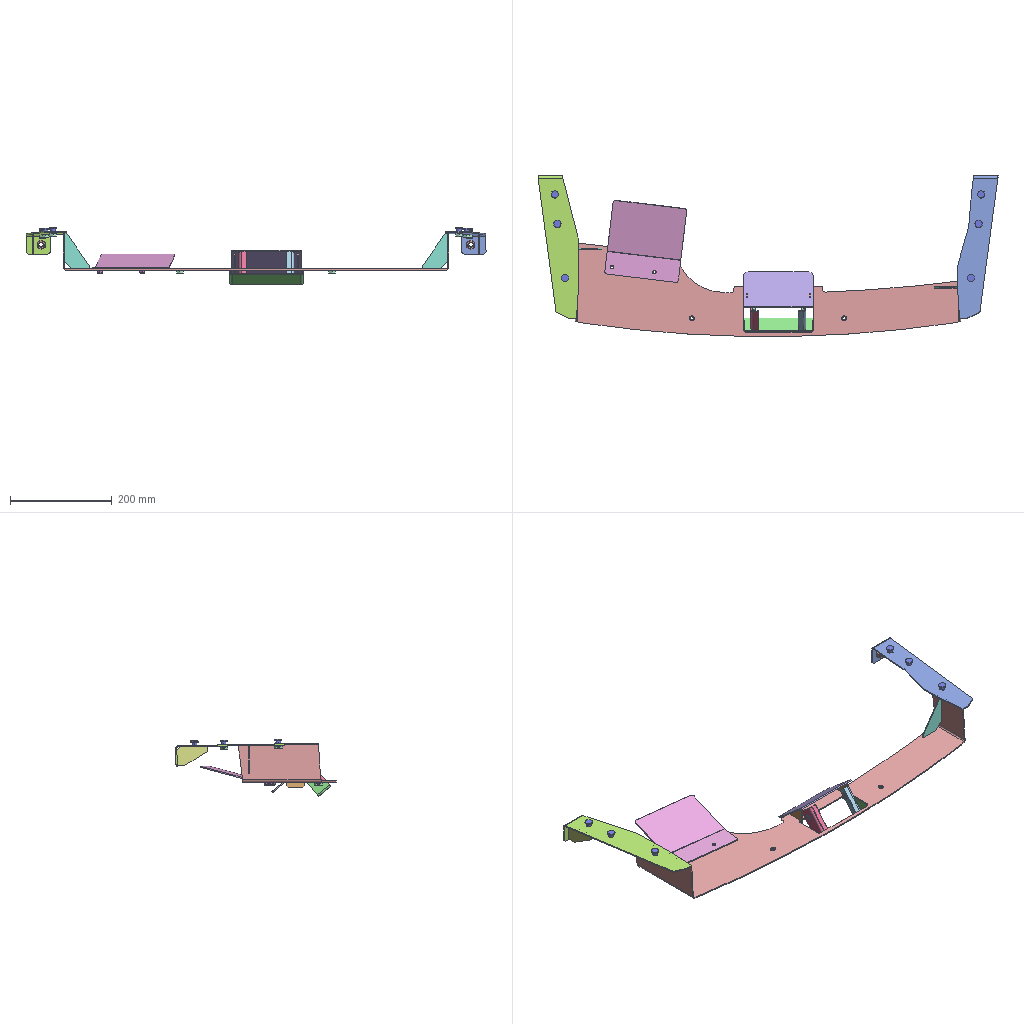Assembly | SolidWorks | 14 different items | 34 placed | box 906 x 316 x 113 mm
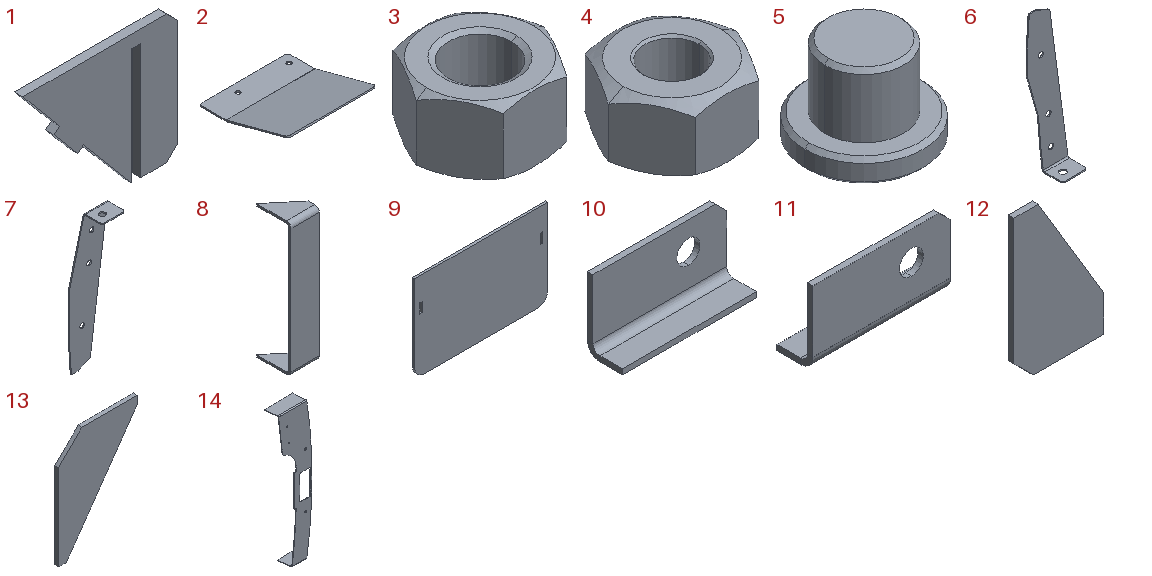Parts list (item | quantity | size | volume | features):
1 | x2 | 42 x 2.3 x 35 mm | 2038 mm3 | features FlatPattern 1, SMBaseFlange 1, SheetMetal 1
2 | x1 | 146 x 146.5 x 29.223 mm | 50041 mm3 | features Fillet 1, FlatPattern 1, ICE 1, SMBaseFlange 1, SheetMetal 1
3 | x12 | 27.713 x 24 x 14.8 mm | 5071 mm3 | features RevCut 2, Chamfer 1, Extrusion 1, LPattern 1
4 | x2 | 11.547 x 10 x 5.7 mm | 373.519 mm3 | features RevCut 4, Chamfer 2, Boss 1, Extrusion 1, LPattern 1
5 | x6 | 15 x 15 x 11 mm | 1143 mm3 | features Chamfer 1, Revolution 1
6 | x1 | 79.693 x 40 x 281.5 mm | 34078 mm3 | features ICE 2, Fillet 1, FlatPattern 1, SMBaseFlange 1, SheetMetal 1
7 | x1 | 79.693 x 40 x 281.5 mm | 37572 mm3 | features ICE 2, Fillet 1, FlatPattern 1, SMBaseFlange 1, SheetMetal 1
8 | x1 | 31 x 37.5 x 145 mm | 13281 mm3 | features FlatPattern 1, ICE 1, SMBaseFlange 1, SheetMetal 1
9 | x1 | 137 x 2.3 x 90 mm | 28143 mm3 | features FlatPattern 1, SMBaseFlange 1, SheetMetal 1
10 | x1 | 57.5 x 15 x 31 mm | 5334 mm3 | features Chamfer 1, FlatPattern 1, ICE 1, SMBaseFlange 1, SheetMetal 1
11 | x1 | 57.5 x 15 x 31 mm | 5334 mm3 | features Chamfer 1, FlatPattern 1, ICE 1, SMBaseFlange 1, SheetMetal 1
12 | x2 | 37 x 2.3 x 60 mm | 3635 mm3 | features FlatPattern 1, SMBaseFlange 1, SheetMetal 1
13 | x2 | 50 x 2.3 x 69.5 mm | 4396 mm3 | features FlatPattern 1, SMBaseFlange 1, SheetMetal 1
14 | x1 | 193.5 x 74.3 x 759.6 mm | 208210 mm3 | features ICE 7, FlatPattern 1, SMBaseFlange 1, SheetMetal 1
Mates (type | each side: item.copy, entity, surface, feature):
Coincident | 14.1 face plane Cut-Extrude3 | 6.1 face plane Base-Flange1
Coincident | 14.1 edge | 6.1 edge
Coincident | 14.1 edge | 6.1 vertex
Parallel | 14.1 face plane Base-Flange1 | 6.1 face plane Base-Flange1
Coincident | 14.1 face plane Cut-Extrude3 | 7.1 face plane Base-Flange1
Coincident | 14.1 edge | 7.1 edge
Coincident | 14.1 edge | 7.1 vertex
Parallel | 14.1 face plane Base-Flange1 | 7.1 face plane Base-Flange1
Coincident | 14.1 face plane Base-Flange1 | 2.1 face plane Base-Flange1
Concentric | 14.1 face cylinder Cut-Extrude4 | 2.1 face cylinder Cut-Extrude1 | 2 times
Coincident | 14.1 face plane Base-Flange1 | 13.1 face plane Base-Flange1 | 2 times
DistanceDim | 13.1 face plane Base-Flange1 | 14.1 edge
Coincident | 14.1 face plane Base-Flange1 | 13.2 face plane Base-Flange1 | 2 times
DistanceDim | 13.2 face plane Base-Flange1 | 13.1 face plane Base-Flange1
Coincident | 14.1 face plane Cut-Extrude4 | 1.1 face plane Base-Flange1
Coincident | 14.1 face plane Base-Flange1 | 1.1 face plane Base-Flange1
DistanceDim | 1.1 face plane Base-Flange1 | 14.1 face plane Cut-Extrude4
Coincident | 14.1 face plane Cut-Extrude4 | 1.2 face plane Base-Flange1
Coincident | 14.1 face plane Base-Flange1 | 1.2 face plane Base-Flange1
DistanceDim | 14.1 face plane Cut-Extrude4 | 1.2 face plane Base-Flange1
Coincident | 1.1 face plane Base-Flange1 | 9.1 face plane Base-Flange1
Coincident | 1.2 face plane Base-Flange1 | 9.1 face plane Base-Flange1 | 2 times
Coincident | 14.1 face plane Base-Flange1 | 8.1 face plane Cut-Extrude1
DistanceDim | 8.1 face plane Base-Flange1 | 14.1 face plane Cut-Extrude4
DistanceDim | 14.1 face plane Cut-Extrude4 | 8.1 edge
Coincident | 8.1 face plane Base-Flange1 | 11.1 face plane Base-Flange1 | 2 times
DistanceDim | 11.1 face plane Base-Flange1 | 8.1 face plane Base-Flange1
Coincident | 8.1 face plane Base-Flange1 | 10.1 face plane Base-Flange1 | 2 times
DistanceDim | 10.1 face plane Base-Flange1 | 11.1 face plane Base-Flange1
Coincident | 7.1 face plane Base-Flange1 | 12.1 face plane Base-Flange1 | 2 times
DistanceDim | 7.1 face plane Cut-Extrude1 | 12.1 face plane Base-Flange1
Coincident | 6.1 face plane Base-Flange1 | 12.2 face plane Base-Flange1 | 2 times
DistanceDim | 6.1 face plane Cut-Extrude1 | 12.2 face plane Base-Flange1
Concentric | 14.1 face cylinder Cut-Extrude4 | 4.1 face cone EndChamfer1
Coincident | 14.1 face plane Base-Flange1 | 4.1 face plane BaseNut
Concentric | 14.1 face cylinder Cut-Extrude4 | 4.2 face cone EndChamfer1
Coincident | 14.1 face plane Base-Flange1 | 4.2 face plane BaseNut
Concentric | 14.1 face cylinder Cut-Extrude4 | 3.1 face cone EndChamfer
Coincident | 14.1 face plane Base-Flange1 | 3.1 face plane BaseNut
Concentric | 14.1 face cylinder Cut-Extrude4 | 3.2 face cone EndChamfer
Coincident | 14.1 face plane Base-Flange1 | 3.2 face plane BaseNut
Concentric | 7.1 face cylinder Cut-Extrude1 | 3.3 face cone EndChamfer
Coincident | 7.1 face plane Base-Flange1 | 3.3 face plane BaseNut
Concentric | 7.1 face cylinder Cut-Extrude1 | 3.4 face cone EndChamfer
Coincident | 7.1 face plane Base-Flange1 | 3.4 face plane BaseNut
Concentric | 7.1 face cylinder Cut-Extrude1 | 3.5 face cone EndChamfer
Coincident | 7.1 face plane Base-Flange1 | 3.5 face plane BaseNut
Concentric | 6.1 face cylinder Cut-Extrude1 | 3.6 face cone EndChamfer
Coincident | 6.1 face plane Base-Flange1 | 3.6 face plane BaseNut
Concentric | 6.1 face cylinder Cut-Extrude1 | 3.7 face cone EndChamfer
Coincident | 6.1 face plane Base-Flange1 | 3.7 face plane BaseNut
Concentric | 6.1 face cylinder Cut-Extrude1 | 3.8 face cone EndChamfer
Coincident | 6.1 face plane Base-Flange1 | 3.8 face plane BaseNut
Concentric | 6.1 face cylinder Cut-Extrude2 | 3.9 face cone EndChamfer
Coincident | 6.1 face plane Base-Flange1 | 3.9 face plane BaseNut
Concentric | 7.1 face cylinder Cut-Extrude2 | 3.10 face cone EndChamfer
Coincident | 7.1 face plane Base-Flange1 | 3.10 face plane BaseNut
Concentric | 10.1 face cylinder Cut-Extrude1 | 3.11 face cone EndChamfer
Coincident | 10.1 face plane Base-Flange1 | 3.11 face plane BaseNut
Concentric | 11.1 face cylinder Cut-Extrude1 | 3.12 face cone EndChamfer
Coincident | 11.1 face plane Base-Flange1 | 3.12 face plane BaseNut
Parallel | 10.1 face plane Base-Flange1 | 3.11 face plane BaseNut